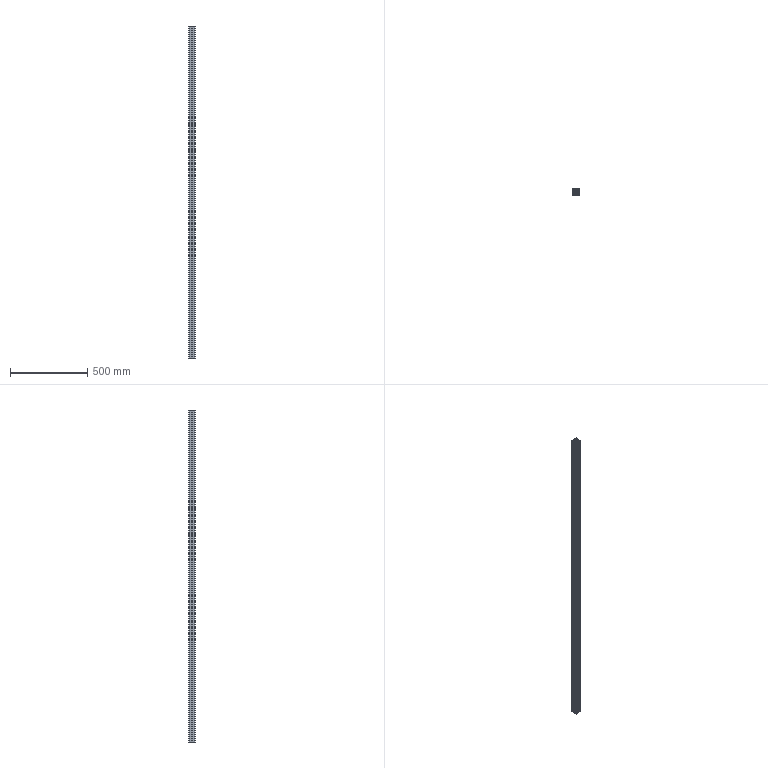Part | SolidWorks | features BaseBody 1, HoleWzd 1, MoveFace 1 | 1 solid | 179 faces | box 40 x 40 x 2154 mm | volume 1154336 mm3 | plane 130 | cylinder 49 | commonest cylinder face diameters 0.6 x24 2 x8 10 x8 6.8 x5 3 x4